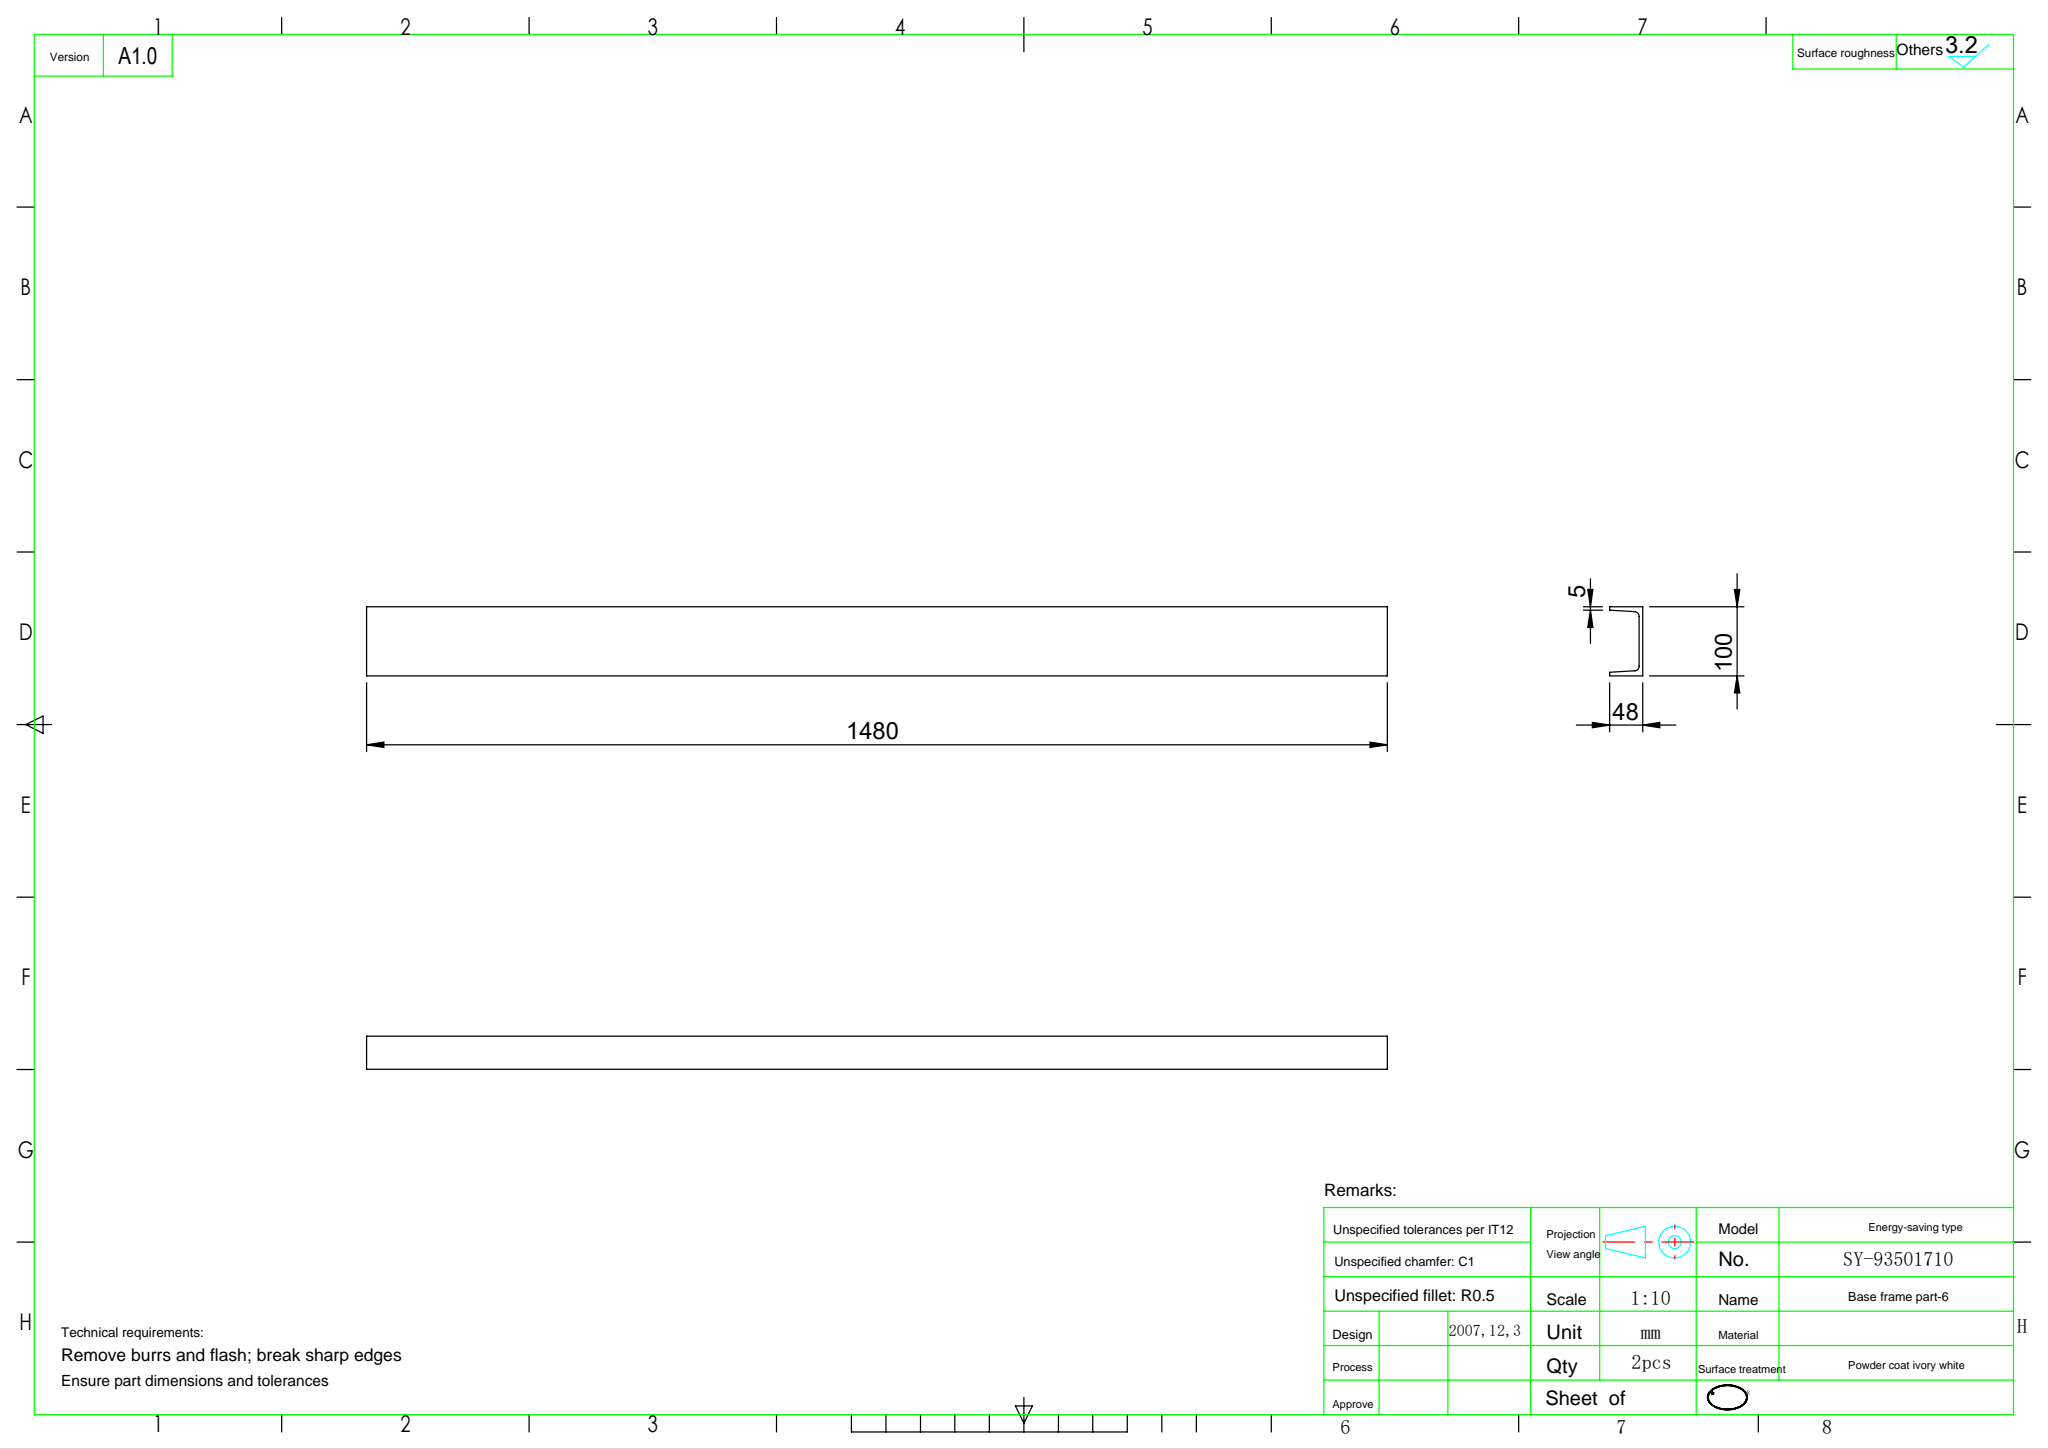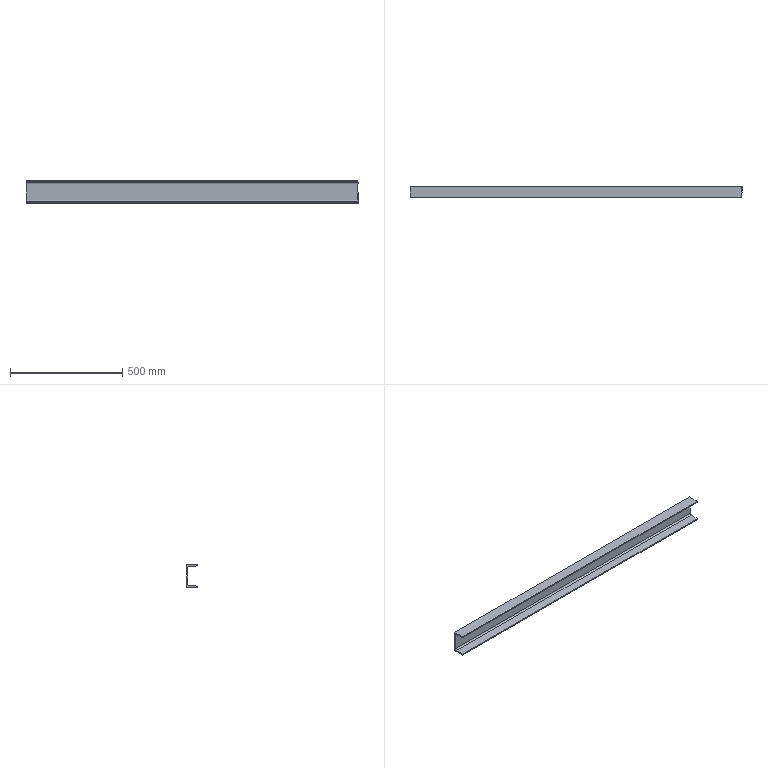Part | SolidWorks | features BaseBody 1, Fillet 1, ICE 1, MoveFace 1 | 1 solid | 12 faces | box 1480 x 48 x 100 mm | volume 1562650 mm3 | plane 10 | cylinder 2 | commonest cylinder face diameters 14 x2
STEP:
#1=CARTESIAN_POINT('',(-1005.,50.,1420.));
#2=VERTEX_POINT('',#1);
#3=CARTESIAN_POINT('',(-1005.,50.,1320.));
#4=VERTEX_POINT('',#3);
#5=CARTESIAN_POINT('',(-1005.,50.,833.715));
#6=DIRECTION('',(0.,0.,-1.));
#7=VECTOR('',#6,1000.);
#8=LINE('',#5,#7);
#9=EDGE_CURVE('',#2,#4,#8,.T.);
#10=ORIENTED_EDGE('',*,*,#9,.F.);
#11=CARTESIAN_POINT('',(475.,50.,1420.));
#12=VERTEX_POINT('',#11);
#13=CARTESIAN_POINT('',(-875.,50.,1420.));
#14=DIRECTION('',(1.,0.,0.));
#15=VECTOR('',#14,1000.);
#16=LINE('',#13,#15);
#17=EDGE_CURVE('',#2,#12,#16,.T.);
#18=ORIENTED_EDGE('',*,*,#17,.T.);
#19=CARTESIAN_POINT('',(475.,50.,1320.));
#20=VERTEX_POINT('',#19);
#21=CARTESIAN_POINT('',(475.,50.,1370.));
#22=DIRECTION('',(0.,0.,-1.));
#23=VECTOR('',#22,1000.);
#24=LINE('',#21,#23);
#25=EDGE_CURVE('',#12,#20,#24,.T.);
#26=ORIENTED_EDGE('',*,*,#25,.T.);
#27=CARTESIAN_POINT('',(-875.,50.,1320.));
#28=DIRECTION('',(-1.,0.,0.));
#29=VECTOR('',#28,1000.);
#30=LINE('',#27,#29);
#31=EDGE_CURVE('',#20,#4,#30,.T.);
#32=ORIENTED_EDGE('',*,*,#31,.T.);
#33=EDGE_LOOP('',(#10,#18,#26,#32));
#34=FACE_OUTER_BOUND('',#33,.T.);
#35=CARTESIAN_POINT('',(-1759.,50.,1317.956));
#36=DIRECTION('',(0.,1.,0.));
#37=DIRECTION('',(0.,0.,1.));
#38=AXIS2_PLACEMENT_3D('',#35,#36,#37);
#39=PLANE('',#38);
#40=ADVANCED_FACE('',(#34),#39,.T.);
#41=CARTESIAN_POINT('',(-1005.,2.,1320.));
#42=VERTEX_POINT('',#41);
#43=CARTESIAN_POINT('',(-1005.,-0.04434,1320.));
#44=DIRECTION('',(0.,-1.,0.));
#45=VECTOR('',#44,1000.);
#46=LINE('',#43,#45);
#47=EDGE_CURVE('',#4,#42,#46,.T.);
#48=ORIENTED_EDGE('',*,*,#47,.F.);
#49=ORIENTED_EDGE('',*,*,#31,.F.);
#50=CARTESIAN_POINT('',(475.,2.,1320.));
#51=VERTEX_POINT('',#50);
#52=CARTESIAN_POINT('',(475.,26.,1320.));
#53=DIRECTION('',(0.,-1.,0.));
#54=VECTOR('',#53,1000.);
#55=LINE('',#52,#54);
#56=EDGE_CURVE('',#20,#51,#55,.T.);
#57=ORIENTED_EDGE('',*,*,#56,.T.);
#58=CARTESIAN_POINT('',(-875.,2.,1320.));
#59=DIRECTION('',(-1.,0.,0.));
#60=VECTOR('',#59,1000.);
#61=LINE('',#58,#60);
#62=EDGE_CURVE('',#51,#42,#61,.T.);
#63=ORIENTED_EDGE('',*,*,#62,.T.);
#64=EDGE_LOOP('',(#48,#49,#57,#63));
#65=FACE_OUTER_BOUND('',#64,.T.);
#66=CARTESIAN_POINT('',(-1759.,-0.04434,1320.));
#67=DIRECTION('',(0.,0.,-1.));
#68=DIRECTION('',(0.,1.,0.));
#69=AXIS2_PLACEMENT_3D('',#66,#67,#68);
#70=PLANE('',#69);
#71=ADVANCED_FACE('',(#65),#70,.T.);
#72=CARTESIAN_POINT('',(-1005.,2.,1325.));
#73=VERTEX_POINT('',#72);
#74=CARTESIAN_POINT('',(-1005.,2.,1327.044));
#75=DIRECTION('',(0.,0.,1.));
#76=VECTOR('',#75,1000.);
#77=LINE('',#74,#76);
#78=EDGE_CURVE('',#42,#73,#77,.T.);
#79=ORIENTED_EDGE('',*,*,#78,.F.);
#80=ORIENTED_EDGE('',*,*,#62,.F.);
#81=CARTESIAN_POINT('',(475.,2.,1325.));
#82=VERTEX_POINT('',#81);
#83=CARTESIAN_POINT('',(475.,2.,1322.5));
#84=DIRECTION('',(0.,0.,1.));
#85=VECTOR('',#84,1000.);
#86=LINE('',#83,#85);
#87=EDGE_CURVE('',#51,#82,#86,.T.);
#88=ORIENTED_EDGE('',*,*,#87,.T.);
#89=CARTESIAN_POINT('',(-875.,2.,1325.));
#90=DIRECTION('',(-1.,0.,0.));
#91=VECTOR('',#90,1000.);
#92=LINE('',#89,#91);
#93=EDGE_CURVE('',#82,#73,#92,.T.);
#94=ORIENTED_EDGE('',*,*,#93,.T.);
#95=EDGE_LOOP('',(#79,#80,#88,#94));
#96=FACE_OUTER_BOUND('',#95,.T.);
#97=CARTESIAN_POINT('',(-1759.,2.,1327.044));
#98=DIRECTION('',(0.,-1.,0.));
#99=DIRECTION('',(0.,0.,-1.));
#100=AXIS2_PLACEMENT_3D('',#97,#98,#99);
#101=PLANE('',#100);
#102=ADVANCED_FACE('',(#96),#101,.T.);
#103=CARTESIAN_POINT('',(-1005.,38.406,1327.117));
#104=VERTEX_POINT('',#103);
#105=CARTESIAN_POINT('',(-1005.,47.041,1327.619));
#106=DIRECTION('',(0.,0.9983,0.05804));
#107=VECTOR('',#106,1000.);
#108=LINE('',#105,#107);
#109=EDGE_CURVE('',#73,#104,#108,.T.);
#110=ORIENTED_EDGE('',*,*,#109,.F.);
#111=ORIENTED_EDGE('',*,*,#93,.F.);
#112=CARTESIAN_POINT('',(475.,38.406,1327.117));
#113=VERTEX_POINT('',#112);
#114=CARTESIAN_POINT('',(475.,23.5,1326.25));
#115=DIRECTION('',(0.,0.9983,0.05804));
#116=VECTOR('',#115,1000.);
#117=LINE('',#114,#116);
#118=EDGE_CURVE('',#82,#113,#117,.T.);
#119=ORIENTED_EDGE('',*,*,#118,.T.);
#120=CARTESIAN_POINT('',(-1725.,38.406,1327.117));
#121=DIRECTION('',(-1.,0.,0.));
#122=VECTOR('',#121,1000.);
#123=LINE('',#120,#122);
#124=EDGE_CURVE('',#113,#104,#123,.T.);
#125=ORIENTED_EDGE('',*,*,#124,.T.);
#126=EDGE_LOOP('',(#110,#111,#119,#125));
#127=FACE_OUTER_BOUND('',#126,.T.);
#128=CARTESIAN_POINT('',(-1759.,47.041,1327.619));
#129=DIRECTION('',(0.,-0.05804,0.9983));
#130=DIRECTION('',(0.,-0.9983,-0.05804));
#131=AXIS2_PLACEMENT_3D('',#128,#129,#130);
#132=PLANE('',#131);
#133=ADVANCED_FACE('',(#127),#132,.T.);
#134=CARTESIAN_POINT('',(-1005.,45.,1334.105));
#135=VERTEX_POINT('',#134);
#136=CARTESIAN_POINT('',(-1005.,45.,1405.895));
#137=VERTEX_POINT('',#136);
#138=CARTESIAN_POINT('',(-1005.,45.,1414.544));
#139=DIRECTION('',(0.,0.,1.));
#140=VECTOR('',#139,1000.);
#141=LINE('',#138,#140);
#142=EDGE_CURVE('',#135,#137,#141,.T.);
#143=ORIENTED_EDGE('',*,*,#142,.F.);
#144=CARTESIAN_POINT('',(475.,45.,1334.105));
#145=VERTEX_POINT('',#144);
#146=CARTESIAN_POINT('',(475.,45.,1334.105));
#147=DIRECTION('',(1.,0.,0.));
#148=VECTOR('',#147,1000.);
#149=LINE('',#146,#148);
#150=EDGE_CURVE('',#135,#145,#149,.T.);
#151=ORIENTED_EDGE('',*,*,#150,.T.);
#152=CARTESIAN_POINT('',(475.,45.,1405.895));
#153=VERTEX_POINT('',#152);
#154=CARTESIAN_POINT('',(475.,45.,1370.));
#155=DIRECTION('',(0.,0.,1.));
#156=VECTOR('',#155,1000.);
#157=LINE('',#154,#156);
#158=EDGE_CURVE('',#145,#153,#157,.T.);
#159=ORIENTED_EDGE('',*,*,#158,.T.);
#160=CARTESIAN_POINT('',(-1725.,45.,1405.895));
#161=DIRECTION('',(-1.,0.,0.));
#162=VECTOR('',#161,1000.);
#163=LINE('',#160,#162);
#164=EDGE_CURVE('',#153,#137,#163,.T.);
#165=ORIENTED_EDGE('',*,*,#164,.T.);
#166=EDGE_LOOP('',(#143,#151,#159,#165));
#167=FACE_OUTER_BOUND('',#166,.T.);
#168=CARTESIAN_POINT('',(-1759.,45.,1414.544));
#169=DIRECTION('',(0.,-1.,0.));
#170=DIRECTION('',(0.,0.,-1.));
#171=AXIS2_PLACEMENT_3D('',#168,#169,#170);
#172=PLANE('',#171);
#173=ADVANCED_FACE('',(#167),#172,.T.);
#174=CARTESIAN_POINT('',(-1005.,38.406,1412.883));
#175=VERTEX_POINT('',#174);
#176=CARTESIAN_POINT('',(-1005.,2.,1415.));
#177=VERTEX_POINT('',#176);
#178=CARTESIAN_POINT('',(-1005.,-0.04089,1415.119));
#179=DIRECTION('',(0.,-0.9983,0.05804));
#180=VECTOR('',#179,1000.);
#181=LINE('',#178,#180);
#182=EDGE_CURVE('',#175,#177,#181,.T.);
#183=ORIENTED_EDGE('',*,*,#182,.F.);
#184=CARTESIAN_POINT('',(475.,38.406,1412.883));
#185=VERTEX_POINT('',#184);
#186=CARTESIAN_POINT('',(475.,38.406,1412.883));
#187=DIRECTION('',(1.,0.,0.));
#188=VECTOR('',#187,1000.);
#189=LINE('',#186,#188);
#190=EDGE_CURVE('',#175,#185,#189,.T.);
#191=ORIENTED_EDGE('',*,*,#190,.T.);
#192=CARTESIAN_POINT('',(475.,2.,1415.));
#193=VERTEX_POINT('',#192);
#194=CARTESIAN_POINT('',(475.,23.5,1413.75));
#195=DIRECTION('',(0.,-0.9983,0.05804));
#196=VECTOR('',#195,1000.);
#197=LINE('',#194,#196);
#198=EDGE_CURVE('',#185,#193,#197,.T.);
#199=ORIENTED_EDGE('',*,*,#198,.T.);
#200=CARTESIAN_POINT('',(-875.,2.,1415.));
#201=DIRECTION('',(-1.,0.,0.));
#202=VECTOR('',#201,1000.);
#203=LINE('',#200,#202);
#204=EDGE_CURVE('',#193,#177,#203,.T.);
#205=ORIENTED_EDGE('',*,*,#204,.T.);
#206=EDGE_LOOP('',(#183,#191,#199,#205));
#207=FACE_OUTER_BOUND('',#206,.T.);
#208=CARTESIAN_POINT('',(-1759.,-0.04089,1415.119));
#209=DIRECTION('',(0.,-0.05804,-0.9983));
#210=DIRECTION('',(0.,0.9983,-0.05804));
#211=AXIS2_PLACEMENT_3D('',#208,#209,#210);
#212=PLANE('',#211);
#213=ADVANCED_FACE('',(#207),#212,.T.);
#214=CARTESIAN_POINT('',(-1005.,2.,1420.));
#215=VERTEX_POINT('',#214);
#216=CARTESIAN_POINT('',(-1005.,2.,1422.044));
#217=DIRECTION('',(0.,0.,1.));
#218=VECTOR('',#217,1000.);
#219=LINE('',#216,#218);
#220=EDGE_CURVE('',#177,#215,#219,.T.);
#221=ORIENTED_EDGE('',*,*,#220,.F.);
#222=ORIENTED_EDGE('',*,*,#204,.F.);
#223=CARTESIAN_POINT('',(475.,2.,1420.));
#224=VERTEX_POINT('',#223);
#225=CARTESIAN_POINT('',(475.,2.,1417.5));
#226=DIRECTION('',(0.,0.,1.));
#227=VECTOR('',#226,1000.);
#228=LINE('',#225,#227);
#229=EDGE_CURVE('',#193,#224,#228,.T.);
#230=ORIENTED_EDGE('',*,*,#229,.T.);
#231=CARTESIAN_POINT('',(-875.,2.,1420.));
#232=DIRECTION('',(-1.,0.,0.));
#233=VECTOR('',#232,1000.);
#234=LINE('',#231,#233);
#235=EDGE_CURVE('',#224,#215,#234,.T.);
#236=ORIENTED_EDGE('',*,*,#235,.T.);
#237=EDGE_LOOP('',(#221,#222,#230,#236));
#238=FACE_OUTER_BOUND('',#237,.T.);
#239=CARTESIAN_POINT('',(-1759.,2.,1422.044));
#240=DIRECTION('',(0.,-1.,0.));
#241=DIRECTION('',(0.,0.,-1.));
#242=AXIS2_PLACEMENT_3D('',#239,#240,#241);
#243=PLANE('',#242);
#244=ADVANCED_FACE('',(#238),#243,.T.);
#245=CARTESIAN_POINT('',(-1005.,52.044,1420.));
#246=DIRECTION('',(0.,1.,0.));
#247=VECTOR('',#246,1000.);
#248=LINE('',#245,#247);
#249=EDGE_CURVE('',#215,#2,#248,.T.);
#250=ORIENTED_EDGE('',*,*,#249,.F.);
#251=ORIENTED_EDGE('',*,*,#235,.F.);
#252=CARTESIAN_POINT('',(475.,26.,1420.));
#253=DIRECTION('',(0.,1.,0.));
#254=VECTOR('',#253,1000.);
#255=LINE('',#252,#254);
#256=EDGE_CURVE('',#224,#12,#255,.T.);
#257=ORIENTED_EDGE('',*,*,#256,.T.);
#258=ORIENTED_EDGE('',*,*,#17,.F.);
#259=EDGE_LOOP('',(#250,#251,#257,#258));
#260=FACE_OUTER_BOUND('',#259,.T.);
#261=CARTESIAN_POINT('',(-1759.,52.044,1420.));
#262=DIRECTION('',(0.,0.,1.));
#263=DIRECTION('',(0.,-1.,0.));
#264=AXIS2_PLACEMENT_3D('',#261,#262,#263);
#265=PLANE('',#264);
#266=ADVANCED_FACE('',(#260),#265,.T.);
#267=ORIENTED_EDGE('',*,*,#56,.F.);
#268=ORIENTED_EDGE('',*,*,#25,.F.);
#269=ORIENTED_EDGE('',*,*,#256,.F.);
#270=ORIENTED_EDGE('',*,*,#229,.F.);
#271=ORIENTED_EDGE('',*,*,#198,.F.);
#272=CARTESIAN_POINT('',(475.,38.,1405.895));
#273=DIRECTION('',(-1.,0.,0.));
#274=DIRECTION('',(0.,0.,-1.));
#275=AXIS2_PLACEMENT_3D('',#272,#273,#274);
#276=CIRCLE('',#275,7.);
#277=EDGE_CURVE('',#185,#153,#276,.T.);
#278=ORIENTED_EDGE('',*,*,#277,.T.);
#279=ORIENTED_EDGE('',*,*,#158,.F.);
#280=CARTESIAN_POINT('',(475.,38.,1334.105));
#281=DIRECTION('',(-1.,0.,0.));
#282=DIRECTION('',(0.,0.,-1.));
#283=AXIS2_PLACEMENT_3D('',#280,#281,#282);
#284=CIRCLE('',#283,7.);
#285=EDGE_CURVE('',#145,#113,#284,.T.);
#286=ORIENTED_EDGE('',*,*,#285,.T.);
#287=ORIENTED_EDGE('',*,*,#118,.F.);
#288=ORIENTED_EDGE('',*,*,#87,.F.);
#289=EDGE_LOOP('',(#267,#268,#269,#270,#271,#278,#279,#286,#287,#288));
#290=FACE_OUTER_BOUND('',#289,.T.);
#291=CARTESIAN_POINT('',(475.,-0.04434,1422.044));
#292=DIRECTION('',(1.,0.,0.));
#293=DIRECTION('',(0.,0.,-1.));
#294=AXIS2_PLACEMENT_3D('',#291,#292,#293);
#295=PLANE('',#294);
#296=ADVANCED_FACE('',(#290),#295,.T.);
#297=ORIENTED_EDGE('',*,*,#190,.F.);
#298=CARTESIAN_POINT('',(-1005.,38.,1405.895));
#299=DIRECTION('',(-1.,0.,0.));
#300=DIRECTION('',(0.,0.,-1.));
#301=AXIS2_PLACEMENT_3D('',#298,#299,#300);
#302=CIRCLE('',#301,7.);
#303=EDGE_CURVE('',#175,#137,#302,.T.);
#304=ORIENTED_EDGE('',*,*,#303,.T.);
#305=ORIENTED_EDGE('',*,*,#164,.F.);
#306=ORIENTED_EDGE('',*,*,#277,.F.);
#307=EDGE_LOOP('',(#297,#304,#305,#306));
#308=FACE_OUTER_BOUND('',#307,.T.);
#309=CARTESIAN_POINT('',(-1759.,38.,1405.895));
#310=DIRECTION('',(1.,0.,0.));
#311=DIRECTION('',(0.,0.,-1.));
#312=AXIS2_PLACEMENT_3D('',#309,#310,#311);
#313=CYLINDRICAL_SURFACE('',#312,7.);
#314=ADVANCED_FACE('',(#308),#313,.F.);
#315=ORIENTED_EDGE('',*,*,#150,.F.);
#316=CARTESIAN_POINT('',(-1005.,38.,1334.105));
#317=DIRECTION('',(-1.,0.,0.));
#318=DIRECTION('',(0.,0.,-1.));
#319=AXIS2_PLACEMENT_3D('',#316,#317,#318);
#320=CIRCLE('',#319,7.);
#321=EDGE_CURVE('',#135,#104,#320,.T.);
#322=ORIENTED_EDGE('',*,*,#321,.T.);
#323=ORIENTED_EDGE('',*,*,#124,.F.);
#324=ORIENTED_EDGE('',*,*,#285,.F.);
#325=EDGE_LOOP('',(#315,#322,#323,#324));
#326=FACE_OUTER_BOUND('',#325,.T.);
#327=CARTESIAN_POINT('',(-1759.,38.,1334.105));
#328=DIRECTION('',(1.,0.,0.));
#329=DIRECTION('',(0.,0.,-1.));
#330=AXIS2_PLACEMENT_3D('',#327,#328,#329);
#331=CYLINDRICAL_SURFACE('',#330,7.);
#332=ADVANCED_FACE('',(#326),#331,.F.);
#333=ORIENTED_EDGE('',*,*,#47,.T.);
#334=ORIENTED_EDGE('',*,*,#78,.T.);
#335=ORIENTED_EDGE('',*,*,#109,.T.);
#336=ORIENTED_EDGE('',*,*,#321,.F.);
#337=ORIENTED_EDGE('',*,*,#142,.T.);
#338=ORIENTED_EDGE('',*,*,#303,.F.);
#339=ORIENTED_EDGE('',*,*,#182,.T.);
#340=ORIENTED_EDGE('',*,*,#220,.T.);
#341=ORIENTED_EDGE('',*,*,#249,.T.);
#342=ORIENTED_EDGE('',*,*,#9,.T.);
#343=EDGE_LOOP('',(#333,#334,#335,#336,#337,#338,#339,#340,#341,#342));
#344=FACE_OUTER_BOUND('',#343,.T.);
#345=CARTESIAN_POINT('',(-1005.,-380.,833.715));
#346=DIRECTION('',(1.,0.,0.));
#347=DIRECTION('',(0.,0.,-1.));
#348=AXIS2_PLACEMENT_3D('',#345,#346,#347);
#349=PLANE('',#348);
#350=ADVANCED_FACE('',(#344),#349,.F.);
#351=CLOSED_SHELL('',(#40,#71,#102,#133,#173,#213,#244,#266,#296,#314,#332,#350));
#352=MANIFOLD_SOLID_BREP('',#351);
#353=CARTESIAN_POINT('',(0.,0.,0.));
#354=DIRECTION('',(0.,0.,1.));
#355=DIRECTION('',(1.,0.,0.));
#356=AXIS2_PLACEMENT_3D('',#353,#354,#355);
#357=(LENGTH_UNIT()NAMED_UNIT(*)SI_UNIT(.MILLI.,.METRE.));
#358=UNCERTAINTY_MEASURE_WITH_UNIT(LENGTH_MEASURE(0.00001),#357,'','');
#359=(NAMED_UNIT(*)PLANE_ANGLE_UNIT()SI_UNIT($,.RADIAN.));
#360=(NAMED_UNIT(*)SI_UNIT($,.STERADIAN.)SOLID_ANGLE_UNIT());
#361=(GEOMETRIC_REPRESENTATION_CONTEXT(3)GLOBAL_UNCERTAINTY_ASSIGNED_CONTEXT((#358))GLOBAL_UNIT_ASSIGNED_CONTEXT((#357,#359,#360))REPRESENTATION_CONTEXT('',''));
#362=ADVANCED_BREP_SHAPE_REPRESENTATION('',(#352,#356),#361);